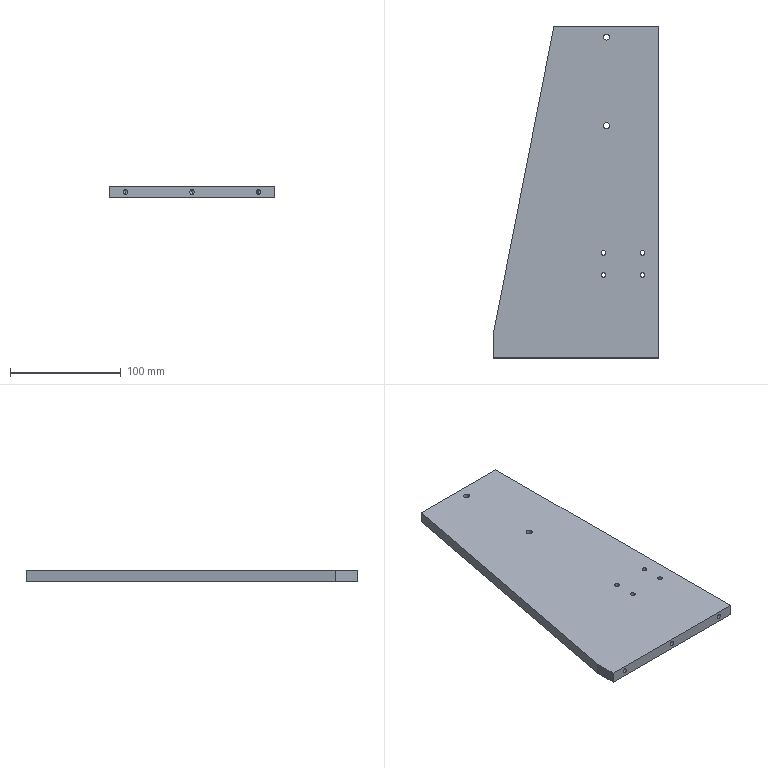Part | STEP file | Grinding bracket upright plate | 1 solid | 54 faces | box 150 x 300 x 10 mm | volume 370376 mm3 | cylinder 30 | cone 17 | plane 7 | commonest cylinder face diameters 4.2 x26 5.5 x4